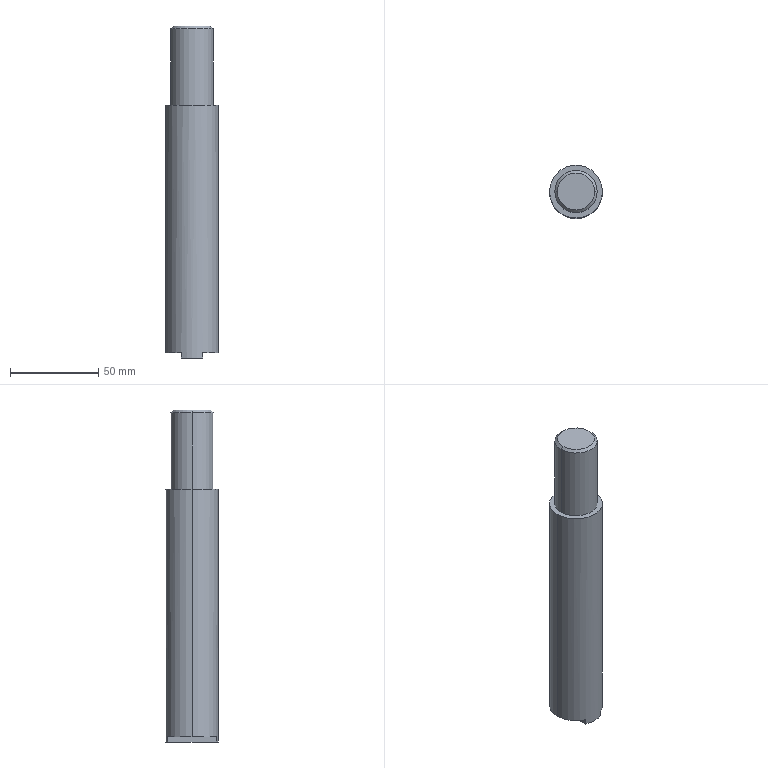Part | SolidWorks | features ICE 2, Chamfer 1, Extrusion 1, HoleWzd 1 | 1 solid | 17 faces | box 30 x 30 x 188 mm | volume 118848 mm3 | plane 7 | cylinder 6 | cone 4 | commonest cylinder face diameters 8.5 x2 24 x2 30 x2
STEP:
#1=CARTESIAN_POINT('',(10.5,0.,185.));
#2=VERTEX_POINT('',#1);
#3=CARTESIAN_POINT('',(-10.5,0.,185.));
#4=VERTEX_POINT('',#3);
#5=CARTESIAN_POINT('',(0.,0.,185.));
#6=DIRECTION('',(0.,0.,1.));
#7=DIRECTION('',(1.,0.,0.));
#8=AXIS2_PLACEMENT_3D('',#5,#6,#7);
#9=CIRCLE('',#8,10.5);
#10=EDGE_CURVE('',#2,#4,#9,.T.);
#11=ORIENTED_EDGE('',*,*,#10,.F.);
#12=CARTESIAN_POINT('',(12.,0.,183.5));
#13=VERTEX_POINT('',#12);
#14=CARTESIAN_POINT('',(10.5,0.,185.));
#15=DIRECTION('',(0.7071,0.,-0.7071));
#16=VECTOR('',#15,1000.);
#17=LINE('',#14,#16);
#18=EDGE_CURVE('',#2,#13,#17,.T.);
#19=ORIENTED_EDGE('',*,*,#18,.T.);
#20=CARTESIAN_POINT('',(-12.,0.,183.5));
#21=VERTEX_POINT('',#20);
#22=CARTESIAN_POINT('',(0.,0.,183.5));
#23=DIRECTION('',(0.,0.,-1.));
#24=DIRECTION('',(1.,0.,0.));
#25=AXIS2_PLACEMENT_3D('',#22,#23,#24);
#26=CIRCLE('',#25,12.);
#27=EDGE_CURVE('',#21,#13,#26,.T.);
#28=ORIENTED_EDGE('',*,*,#27,.F.);
#29=CARTESIAN_POINT('',(-10.5,0.,185.));
#30=DIRECTION('',(-0.7071,0.,-0.7071));
#31=VECTOR('',#30,1000.);
#32=LINE('',#29,#31);
#33=EDGE_CURVE('',#4,#21,#32,.T.);
#34=ORIENTED_EDGE('',*,*,#33,.F.);
#35=EDGE_LOOP('',(#11,#19,#28,#34));
#36=FACE_OUTER_BOUND('',#35,.T.);
#37=CARTESIAN_POINT('',(0.,0.,185.));
#38=DIRECTION('',(0.,0.,-1.));
#39=DIRECTION('',(-1.,0.,0.));
#40=AXIS2_PLACEMENT_3D('',#37,#38,#39);
#41=CONICAL_SURFACE('',#40,10.5,0.7854);
#42=ADVANCED_FACE('',(#36),#41,.T.);
#43=CARTESIAN_POINT('',(4.25,0.,21.5));
#44=VERTEX_POINT('',#43);
#45=CARTESIAN_POINT('',(-4.25,0.,21.5));
#46=VERTEX_POINT('',#45);
#47=CARTESIAN_POINT('',(0.,0.,21.5));
#48=DIRECTION('',(0.,0.,-1.));
#49=DIRECTION('',(-1.,0.,0.));
#50=AXIS2_PLACEMENT_3D('',#47,#48,#49);
#51=CIRCLE('',#50,4.25);
#52=EDGE_CURVE('',#44,#46,#51,.T.);
#53=ORIENTED_EDGE('',*,*,#52,.F.);
#54=CARTESIAN_POINT('',(4.25,0.,-3.));
#55=VERTEX_POINT('',#54);
#56=CARTESIAN_POINT('',(4.25,0.,-3.));
#57=DIRECTION('',(0.,0.,-1.));
#58=VECTOR('',#57,1000.);
#59=LINE('',#56,#58);
#60=EDGE_CURVE('',#44,#55,#59,.T.);
#61=ORIENTED_EDGE('',*,*,#60,.T.);
#62=CARTESIAN_POINT('',(-4.25,0.,-3.));
#63=VERTEX_POINT('',#62);
#64=CARTESIAN_POINT('',(0.,0.,-3.));
#65=DIRECTION('',(0.,0.,-1.));
#66=DIRECTION('',(-1.,0.,0.));
#67=AXIS2_PLACEMENT_3D('',#64,#65,#66);
#68=CIRCLE('',#67,4.25);
#69=EDGE_CURVE('',#55,#63,#68,.T.);
#70=ORIENTED_EDGE('',*,*,#69,.T.);
#71=CARTESIAN_POINT('',(-4.25,0.,-3.));
#72=DIRECTION('',(0.,0.,-1.));
#73=VECTOR('',#72,1000.);
#74=LINE('',#71,#73);
#75=EDGE_CURVE('',#46,#63,#74,.T.);
#76=ORIENTED_EDGE('',*,*,#75,.F.);
#77=EDGE_LOOP('',(#53,#61,#70,#76));
#78=FACE_OUTER_BOUND('',#77,.T.);
#79=CARTESIAN_POINT('',(0.,0.,-3.));
#80=DIRECTION('',(0.,0.,-1.));
#81=DIRECTION('',(-1.,0.,0.));
#82=AXIS2_PLACEMENT_3D('',#79,#80,#81);
#83=CYLINDRICAL_SURFACE('',#82,4.25);
#84=ADVANCED_FACE('',(#78),#83,.F.);
#85=CARTESIAN_POINT('',(0.,0.,24.054));
#86=VERTEX_POINT('',#85);
#87=CARTESIAN_POINT('',(-4.25,0.,21.5));
#88=DIRECTION('',(-0.8572,0.,-0.515));
#89=VECTOR('',#88,1000.);
#90=LINE('',#87,#89);
#91=EDGE_CURVE('',#86,#46,#90,.T.);
#92=ORIENTED_EDGE('',*,*,#91,.F.);
#93=CARTESIAN_POINT('',(4.25,0.,21.5));
#94=DIRECTION('',(0.8572,0.,-0.515));
#95=VECTOR('',#94,1000.);
#96=LINE('',#93,#95);
#97=EDGE_CURVE('',#86,#44,#96,.T.);
#98=ORIENTED_EDGE('',*,*,#97,.T.);
#99=ORIENTED_EDGE('',*,*,#52,.T.);
#100=EDGE_LOOP('',(#92,#98,#99));
#101=FACE_OUTER_BOUND('',#100,.T.);
#102=CARTESIAN_POINT('',(0.,0.,21.5));
#103=DIRECTION('',(0.,0.,-1.));
#104=DIRECTION('',(-1.,0.,0.));
#105=AXIS2_PLACEMENT_3D('',#102,#103,#104);
#106=CONICAL_SURFACE('',#105,4.25,1.03);
#107=ADVANCED_FACE('',(#101),#106,.F.);
#108=ORIENTED_EDGE('',*,*,#27,.T.);
#109=CARTESIAN_POINT('',(12.,0.,140.));
#110=VERTEX_POINT('',#109);
#111=CARTESIAN_POINT('',(12.,0.,185.));
#112=DIRECTION('',(0.,0.,-1.));
#113=VECTOR('',#112,1000.);
#114=LINE('',#111,#113);
#115=EDGE_CURVE('',#13,#110,#114,.T.);
#116=ORIENTED_EDGE('',*,*,#115,.T.);
#117=CARTESIAN_POINT('',(-12.,0.,140.));
#118=VERTEX_POINT('',#117);
#119=CARTESIAN_POINT('',(0.,0.,140.));
#120=DIRECTION('',(0.,0.,1.));
#121=DIRECTION('',(1.,0.,0.));
#122=AXIS2_PLACEMENT_3D('',#119,#120,#121);
#123=CIRCLE('',#122,12.);
#124=EDGE_CURVE('',#110,#118,#123,.T.);
#125=ORIENTED_EDGE('',*,*,#124,.T.);
#126=CARTESIAN_POINT('',(-12.,0.,185.));
#127=DIRECTION('',(0.,0.,-1.));
#128=VECTOR('',#127,1000.);
#129=LINE('',#126,#128);
#130=EDGE_CURVE('',#21,#118,#129,.T.);
#131=ORIENTED_EDGE('',*,*,#130,.F.);
#132=EDGE_LOOP('',(#108,#116,#125,#131));
#133=FACE_OUTER_BOUND('',#132,.T.);
#134=CARTESIAN_POINT('',(0.,0.,185.));
#135=DIRECTION('',(0.,0.,-1.));
#136=DIRECTION('',(-1.,0.,0.));
#137=AXIS2_PLACEMENT_3D('',#134,#135,#136);
#138=CYLINDRICAL_SURFACE('',#137,12.);
#139=ADVANCED_FACE('',(#133),#138,.T.);
#140=CARTESIAN_POINT('',(15.,0.,140.));
#141=VERTEX_POINT('',#140);
#142=CARTESIAN_POINT('',(-15.,0.,140.));
#143=VERTEX_POINT('',#142);
#144=CARTESIAN_POINT('',(0.,0.,140.));
#145=DIRECTION('',(0.,0.,1.));
#146=DIRECTION('',(1.,0.,0.));
#147=AXIS2_PLACEMENT_3D('',#144,#145,#146);
#148=CIRCLE('',#147,15.);
#149=EDGE_CURVE('',#141,#143,#148,.T.);
#150=ORIENTED_EDGE('',*,*,#149,.F.);
#151=CARTESIAN_POINT('',(15.,0.,0.));
#152=VERTEX_POINT('',#151);
#153=CARTESIAN_POINT('',(15.,0.,140.));
#154=DIRECTION('',(0.,0.,-1.));
#155=VECTOR('',#154,1000.);
#156=LINE('',#153,#155);
#157=EDGE_CURVE('',#141,#152,#156,.T.);
#158=ORIENTED_EDGE('',*,*,#157,.T.);
#159=CARTESIAN_POINT('',(6.,13.748,0.));
#160=VERTEX_POINT('',#159);
#161=CARTESIAN_POINT('',(0.,0.,0.));
#162=DIRECTION('',(0.,0.,1.));
#163=DIRECTION('',(1.,0.,0.));
#164=AXIS2_PLACEMENT_3D('',#161,#162,#163);
#165=CIRCLE('',#164,15.);
#166=EDGE_CURVE('',#152,#160,#165,.T.);
#167=ORIENTED_EDGE('',*,*,#166,.T.);
#168=CARTESIAN_POINT('',(6.,13.748,-3.));
#169=VERTEX_POINT('',#168);
#170=CARTESIAN_POINT('',(6.,13.748,-3.));
#171=DIRECTION('',(0.,0.,1.));
#172=VECTOR('',#171,1000.);
#173=LINE('',#170,#172);
#174=EDGE_CURVE('',#169,#160,#173,.T.);
#175=ORIENTED_EDGE('',*,*,#174,.F.);
#176=CARTESIAN_POINT('',(-6.,13.748,-3.));
#177=VERTEX_POINT('',#176);
#178=CARTESIAN_POINT('',(0.,0.,-3.));
#179=DIRECTION('',(0.,0.,-1.));
#180=DIRECTION('',(-1.,0.,0.));
#181=AXIS2_PLACEMENT_3D('',#178,#179,#180);
#182=CIRCLE('',#181,15.);
#183=EDGE_CURVE('',#177,#169,#182,.T.);
#184=ORIENTED_EDGE('',*,*,#183,.F.);
#185=CARTESIAN_POINT('',(-6.,13.748,0.));
#186=VERTEX_POINT('',#185);
#187=CARTESIAN_POINT('',(-6.,13.748,-3.));
#188=DIRECTION('',(0.,0.,1.));
#189=VECTOR('',#188,1000.);
#190=LINE('',#187,#189);
#191=EDGE_CURVE('',#177,#186,#190,.T.);
#192=ORIENTED_EDGE('',*,*,#191,.T.);
#193=CARTESIAN_POINT('',(-15.,0.,0.));
#194=VERTEX_POINT('',#193);
#195=CARTESIAN_POINT('',(0.,0.,0.));
#196=DIRECTION('',(0.,0.,1.));
#197=DIRECTION('',(1.,0.,0.));
#198=AXIS2_PLACEMENT_3D('',#195,#196,#197);
#199=CIRCLE('',#198,15.);
#200=EDGE_CURVE('',#186,#194,#199,.T.);
#201=ORIENTED_EDGE('',*,*,#200,.T.);
#202=CARTESIAN_POINT('',(-15.,0.,140.));
#203=DIRECTION('',(0.,0.,-1.));
#204=VECTOR('',#203,1000.);
#205=LINE('',#202,#204);
#206=EDGE_CURVE('',#143,#194,#205,.T.);
#207=ORIENTED_EDGE('',*,*,#206,.F.);
#208=EDGE_LOOP('',(#150,#158,#167,#175,#184,#192,#201,#207));
#209=FACE_OUTER_BOUND('',#208,.T.);
#210=CARTESIAN_POINT('',(0.,0.,140.));
#211=DIRECTION('',(0.,0.,-1.));
#212=DIRECTION('',(-1.,0.,0.));
#213=AXIS2_PLACEMENT_3D('',#210,#211,#212);
#214=CYLINDRICAL_SURFACE('',#213,15.);
#215=ADVANCED_FACE('',(#209),#214,.T.);
#216=CARTESIAN_POINT('',(-6.,-13.748,0.));
#217=VERTEX_POINT('',#216);
#218=CARTESIAN_POINT('',(-6.,13.748,0.));
#219=DIRECTION('',(0.,1.,0.));
#220=VECTOR('',#219,1000.);
#221=LINE('',#218,#220);
#222=EDGE_CURVE('',#217,#186,#221,.T.);
#223=ORIENTED_EDGE('',*,*,#222,.F.);
#224=CARTESIAN_POINT('',(0.,0.,0.));
#225=DIRECTION('',(0.,0.,1.));
#226=DIRECTION('',(1.,0.,0.));
#227=AXIS2_PLACEMENT_3D('',#224,#225,#226);
#228=CIRCLE('',#227,15.);
#229=EDGE_CURVE('',#194,#217,#228,.T.);
#230=ORIENTED_EDGE('',*,*,#229,.F.);
#231=ORIENTED_EDGE('',*,*,#200,.F.);
#232=EDGE_LOOP('',(#223,#230,#231));
#233=FACE_OUTER_BOUND('',#232,.T.);
#234=CARTESIAN_POINT('',(0.,0.,0.));
#235=DIRECTION('',(0.,0.,1.));
#236=DIRECTION('',(1.,0.,0.));
#237=AXIS2_PLACEMENT_3D('',#234,#235,#236);
#238=PLANE('',#237);
#239=ADVANCED_FACE('',(#233),#238,.F.);
#240=CARTESIAN_POINT('',(6.,-13.748,0.));
#241=VERTEX_POINT('',#240);
#242=CARTESIAN_POINT('',(6.,13.748,0.));
#243=DIRECTION('',(0.,-1.,0.));
#244=VECTOR('',#243,1000.);
#245=LINE('',#242,#244);
#246=EDGE_CURVE('',#160,#241,#245,.T.);
#247=ORIENTED_EDGE('',*,*,#246,.F.);
#248=ORIENTED_EDGE('',*,*,#166,.F.);
#249=CARTESIAN_POINT('',(0.,0.,0.));
#250=DIRECTION('',(0.,0.,1.));
#251=DIRECTION('',(1.,0.,0.));
#252=AXIS2_PLACEMENT_3D('',#249,#250,#251);
#253=CIRCLE('',#252,15.);
#254=EDGE_CURVE('',#241,#152,#253,.T.);
#255=ORIENTED_EDGE('',*,*,#254,.F.);
#256=EDGE_LOOP('',(#247,#248,#255));
#257=FACE_OUTER_BOUND('',#256,.T.);
#258=CARTESIAN_POINT('',(0.,0.,0.));
#259=DIRECTION('',(0.,0.,1.));
#260=DIRECTION('',(1.,0.,0.));
#261=AXIS2_PLACEMENT_3D('',#258,#259,#260);
#262=PLANE('',#261);
#263=ADVANCED_FACE('',(#257),#262,.F.);
#264=CARTESIAN_POINT('',(0.,0.,140.));
#265=DIRECTION('',(0.,0.,1.));
#266=DIRECTION('',(1.,0.,0.));
#267=AXIS2_PLACEMENT_3D('',#264,#265,#266);
#268=CIRCLE('',#267,15.);
#269=EDGE_CURVE('',#143,#141,#268,.T.);
#270=ORIENTED_EDGE('',*,*,#269,.T.);
#271=ORIENTED_EDGE('',*,*,#149,.T.);
#272=EDGE_LOOP('',(#270,#271));
#273=FACE_OUTER_BOUND('',#272,.T.);
#274=CARTESIAN_POINT('',(0.,0.,140.));
#275=DIRECTION('',(0.,0.,1.));
#276=DIRECTION('',(1.,0.,0.));
#277=AXIS2_PLACEMENT_3D('',#274,#275,#276);
#278=CIRCLE('',#277,12.);
#279=EDGE_CURVE('',#118,#110,#278,.T.);
#280=ORIENTED_EDGE('',*,*,#279,.F.);
#281=ORIENTED_EDGE('',*,*,#124,.F.);
#282=EDGE_LOOP('',(#280,#281));
#283=FACE_BOUND('',#282,.T.);
#284=CARTESIAN_POINT('',(0.,0.,140.));
#285=DIRECTION('',(0.,0.,1.));
#286=DIRECTION('',(1.,0.,0.));
#287=AXIS2_PLACEMENT_3D('',#284,#285,#286);
#288=PLANE('',#287);
#289=ADVANCED_FACE('',(#273,#283),#288,.T.);
#290=ORIENTED_EDGE('',*,*,#157,.F.);
#291=ORIENTED_EDGE('',*,*,#269,.F.);
#292=ORIENTED_EDGE('',*,*,#206,.T.);
#293=ORIENTED_EDGE('',*,*,#229,.T.);
#294=CARTESIAN_POINT('',(-6.,-13.748,-3.));
#295=VERTEX_POINT('',#294);
#296=CARTESIAN_POINT('',(-6.,-13.748,-3.));
#297=DIRECTION('',(0.,0.,1.));
#298=VECTOR('',#297,1000.);
#299=LINE('',#296,#298);
#300=EDGE_CURVE('',#295,#217,#299,.T.);
#301=ORIENTED_EDGE('',*,*,#300,.F.);
#302=CARTESIAN_POINT('',(6.,-13.748,-3.));
#303=VERTEX_POINT('',#302);
#304=CARTESIAN_POINT('',(0.,0.,-3.));
#305=DIRECTION('',(0.,0.,-1.));
#306=DIRECTION('',(-1.,0.,0.));
#307=AXIS2_PLACEMENT_3D('',#304,#305,#306);
#308=CIRCLE('',#307,15.);
#309=EDGE_CURVE('',#303,#295,#308,.T.);
#310=ORIENTED_EDGE('',*,*,#309,.F.);
#311=CARTESIAN_POINT('',(6.,-13.748,-3.));
#312=DIRECTION('',(0.,0.,1.));
#313=VECTOR('',#312,1000.);
#314=LINE('',#311,#313);
#315=EDGE_CURVE('',#303,#241,#314,.T.);
#316=ORIENTED_EDGE('',*,*,#315,.T.);
#317=ORIENTED_EDGE('',*,*,#254,.T.);
#318=EDGE_LOOP('',(#290,#291,#292,#293,#301,#310,#316,#317));
#319=FACE_OUTER_BOUND('',#318,.T.);
#320=CARTESIAN_POINT('',(0.,0.,140.));
#321=DIRECTION('',(0.,0.,-1.));
#322=DIRECTION('',(-1.,0.,0.));
#323=AXIS2_PLACEMENT_3D('',#320,#321,#322);
#324=CYLINDRICAL_SURFACE('',#323,15.);
#325=ADVANCED_FACE('',(#319),#324,.T.);
#326=ORIENTED_EDGE('',*,*,#115,.F.);
#327=CARTESIAN_POINT('',(0.,0.,183.5));
#328=DIRECTION('',(0.,0.,-1.));
#329=DIRECTION('',(1.,0.,0.));
#330=AXIS2_PLACEMENT_3D('',#327,#328,#329);
#331=CIRCLE('',#330,12.);
#332=EDGE_CURVE('',#13,#21,#331,.T.);
#333=ORIENTED_EDGE('',*,*,#332,.T.);
#334=ORIENTED_EDGE('',*,*,#130,.T.);
#335=ORIENTED_EDGE('',*,*,#279,.T.);
#336=EDGE_LOOP('',(#326,#333,#334,#335));
#337=FACE_OUTER_BOUND('',#336,.T.);
#338=CARTESIAN_POINT('',(0.,0.,185.));
#339=DIRECTION('',(0.,0.,-1.));
#340=DIRECTION('',(-1.,0.,0.));
#341=AXIS2_PLACEMENT_3D('',#338,#339,#340);
#342=CYLINDRICAL_SURFACE('',#341,12.);
#343=ADVANCED_FACE('',(#337),#342,.T.);
#344=CARTESIAN_POINT('',(0.,0.,185.));
#345=DIRECTION('',(0.,0.,1.));
#346=DIRECTION('',(1.,0.,0.));
#347=AXIS2_PLACEMENT_3D('',#344,#345,#346);
#348=CIRCLE('',#347,10.5);
#349=EDGE_CURVE('',#4,#2,#348,.T.);
#350=ORIENTED_EDGE('',*,*,#349,.T.);
#351=ORIENTED_EDGE('',*,*,#10,.T.);
#352=EDGE_LOOP('',(#350,#351));
#353=FACE_OUTER_BOUND('',#352,.T.);
#354=CARTESIAN_POINT('',(0.,0.,185.));
#355=DIRECTION('',(0.,0.,1.));
#356=DIRECTION('',(1.,0.,0.));
#357=AXIS2_PLACEMENT_3D('',#354,#355,#356);
#358=PLANE('',#357);
#359=ADVANCED_FACE('',(#353),#358,.T.);
#360=ORIENTED_EDGE('',*,*,#246,.T.);
#361=ORIENTED_EDGE('',*,*,#315,.F.);
#362=CARTESIAN_POINT('',(6.,13.748,-3.));
#363=DIRECTION('',(0.,-1.,0.));
#364=VECTOR('',#363,1000.);
#365=LINE('',#362,#364);
#366=EDGE_CURVE('',#169,#303,#365,.T.);
#367=ORIENTED_EDGE('',*,*,#366,.F.);
#368=ORIENTED_EDGE('',*,*,#174,.T.);
#369=EDGE_LOOP('',(#360,#361,#367,#368));
#370=FACE_OUTER_BOUND('',#369,.T.);
#371=CARTESIAN_POINT('',(6.,13.748,-3.));
#372=DIRECTION('',(-1.,0.,0.));
#373=DIRECTION('',(0.,-1.,0.));
#374=AXIS2_PLACEMENT_3D('',#371,#372,#373);
#375=PLANE('',#374);
#376=ADVANCED_FACE('',(#370),#375,.F.);
#377=ORIENTED_EDGE('',*,*,#222,.T.);
#378=ORIENTED_EDGE('',*,*,#191,.F.);
#379=CARTESIAN_POINT('',(-6.,13.748,-3.));
#380=DIRECTION('',(0.,1.,0.));
#381=VECTOR('',#380,1000.);
#382=LINE('',#379,#381);
#383=EDGE_CURVE('',#295,#177,#382,.T.);
#384=ORIENTED_EDGE('',*,*,#383,.F.);
#385=ORIENTED_EDGE('',*,*,#300,.T.);
#386=EDGE_LOOP('',(#377,#378,#384,#385));
#387=FACE_OUTER_BOUND('',#386,.T.);
#388=CARTESIAN_POINT('',(-6.,13.748,-3.));
#389=DIRECTION('',(1.,0.,0.));
#390=DIRECTION('',(0.,1.,0.));
#391=AXIS2_PLACEMENT_3D('',#388,#389,#390);
#392=PLANE('',#391);
#393=ADVANCED_FACE('',(#387),#392,.F.);
#394=CARTESIAN_POINT('',(0.,0.,-3.));
#395=DIRECTION('',(0.,0.,-1.));
#396=DIRECTION('',(-1.,0.,0.));
#397=AXIS2_PLACEMENT_3D('',#394,#395,#396);
#398=CIRCLE('',#397,4.25);
#399=EDGE_CURVE('',#63,#55,#398,.T.);
#400=ORIENTED_EDGE('',*,*,#399,.F.);
#401=ORIENTED_EDGE('',*,*,#69,.F.);
#402=EDGE_LOOP('',(#400,#401));
#403=FACE_BOUND('',#402,.T.);
#404=ORIENTED_EDGE('',*,*,#183,.T.);
#405=ORIENTED_EDGE('',*,*,#366,.T.);
#406=ORIENTED_EDGE('',*,*,#309,.T.);
#407=ORIENTED_EDGE('',*,*,#383,.T.);
#408=EDGE_LOOP('',(#404,#405,#406,#407));
#409=FACE_OUTER_BOUND('',#408,.T.);
#410=CARTESIAN_POINT('',(0.,0.,-3.));
#411=DIRECTION('',(0.,0.,-1.));
#412=DIRECTION('',(-1.,0.,0.));
#413=AXIS2_PLACEMENT_3D('',#410,#411,#412);
#414=PLANE('',#413);
#415=ADVANCED_FACE('',(#403,#409),#414,.T.);
#416=ORIENTED_EDGE('',*,*,#97,.F.);
#417=ORIENTED_EDGE('',*,*,#91,.T.);
#418=CARTESIAN_POINT('',(0.,0.,21.5));
#419=DIRECTION('',(0.,0.,-1.));
#420=DIRECTION('',(-1.,0.,0.));
#421=AXIS2_PLACEMENT_3D('',#418,#419,#420);
#422=CIRCLE('',#421,4.25);
#423=EDGE_CURVE('',#46,#44,#422,.T.);
#424=ORIENTED_EDGE('',*,*,#423,.T.);
#425=EDGE_LOOP('',(#416,#417,#424));
#426=FACE_OUTER_BOUND('',#425,.T.);
#427=CARTESIAN_POINT('',(0.,0.,21.5));
#428=DIRECTION('',(0.,0.,-1.));
#429=DIRECTION('',(-1.,0.,0.));
#430=AXIS2_PLACEMENT_3D('',#427,#428,#429);
#431=CONICAL_SURFACE('',#430,4.25,1.03);
#432=ADVANCED_FACE('',(#426),#431,.F.);
#433=ORIENTED_EDGE('',*,*,#60,.F.);
#434=ORIENTED_EDGE('',*,*,#423,.F.);
#435=ORIENTED_EDGE('',*,*,#75,.T.);
#436=ORIENTED_EDGE('',*,*,#399,.T.);
#437=EDGE_LOOP('',(#433,#434,#435,#436));
#438=FACE_OUTER_BOUND('',#437,.T.);
#439=CARTESIAN_POINT('',(0.,0.,-3.));
#440=DIRECTION('',(0.,0.,-1.));
#441=DIRECTION('',(-1.,0.,0.));
#442=AXIS2_PLACEMENT_3D('',#439,#440,#441);
#443=CYLINDRICAL_SURFACE('',#442,4.25);
#444=ADVANCED_FACE('',(#438),#443,.F.);
#445=ORIENTED_EDGE('',*,*,#18,.F.);
#446=ORIENTED_EDGE('',*,*,#349,.F.);
#447=ORIENTED_EDGE('',*,*,#33,.T.);
#448=ORIENTED_EDGE('',*,*,#332,.F.);
#449=EDGE_LOOP('',(#445,#446,#447,#448));
#450=FACE_OUTER_BOUND('',#449,.T.);
#451=CARTESIAN_POINT('',(0.,0.,185.));
#452=DIRECTION('',(0.,0.,-1.));
#453=DIRECTION('',(-1.,0.,0.));
#454=AXIS2_PLACEMENT_3D('',#451,#452,#453);
#455=CONICAL_SURFACE('',#454,10.5,0.7854);
#456=ADVANCED_FACE('',(#450),#455,.T.);
#457=CLOSED_SHELL('',(#42,#84,#107,#139,#215,#239,#263,#289,#325,#343,#359,#376,#393,#415,#432,#444,#456));
#458=MANIFOLD_SOLID_BREP('',#457);
#459=CARTESIAN_POINT('',(0.,0.,0.));
#460=DIRECTION('',(0.,0.,1.));
#461=DIRECTION('',(1.,0.,0.));
#462=AXIS2_PLACEMENT_3D('',#459,#460,#461);
#463=(LENGTH_UNIT()NAMED_UNIT(*)SI_UNIT(.MILLI.,.METRE.));
#464=UNCERTAINTY_MEASURE_WITH_UNIT(LENGTH_MEASURE(0.00001),#463,'','');
#465=(NAMED_UNIT(*)PLANE_ANGLE_UNIT()SI_UNIT($,.RADIAN.));
#466=(NAMED_UNIT(*)SI_UNIT($,.STERADIAN.)SOLID_ANGLE_UNIT());
#467=(GEOMETRIC_REPRESENTATION_CONTEXT(3)GLOBAL_UNCERTAINTY_ASSIGNED_CONTEXT((#464))GLOBAL_UNIT_ASSIGNED_CONTEXT((#463,#465,#466))REPRESENTATION_CONTEXT('',''));
#468=ADVANCED_BREP_SHAPE_REPRESENTATION('',(#458,#462),#467);